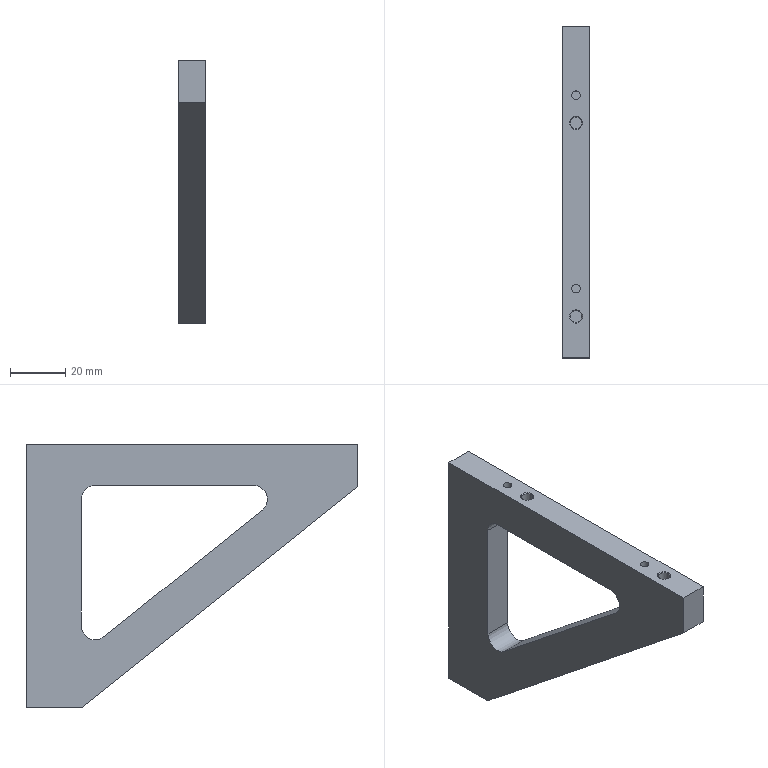Part | STEP file | ROTATION MC_NEW VER-0610_564 | 1 solid | 29 faces | box 10 x 120 x 95.441 mm | volume 51150 mm3 | plane 16 | cylinder 9 | cone 4 | commonest cylinder face diameters 4.2 x4 10 x3 3.03 x2
STEP:
#1=CARTESIAN_POINT('',(-324.569,673.508,-231.532));
#2=VERTEX_POINT('',#1);
#3=CARTESIAN_POINT('',(-322.469,673.508,-231.532));
#4=DIRECTION('',(0.,1.,0.));
#5=DIRECTION('',(-1.,0.,0.));
#6=AXIS2_PLACEMENT_3D('',#3,#4,#5);
#7=CIRCLE('',#6,2.1);
#8=EDGE_CURVE('',#2,#2,#7,.T.);
#9=ORIENTED_EDGE('',*,*,#8,.F.);
#10=CARTESIAN_POINT('',(-324.569,683.208,-231.532));
#11=VERTEX_POINT('',#10);
#12=CARTESIAN_POINT('',(-324.569,688.008,-231.532));
#13=DIRECTION('',(0.,1.,0.));
#14=VECTOR('',#13,2.1);
#15=LINE('',#12,#14);
#16=EDGE_CURVE('',#2,#11,#15,.T.);
#17=ORIENTED_EDGE('',*,*,#16,.T.);
#18=CARTESIAN_POINT('',(-320.369,683.208,-231.532));
#19=VERTEX_POINT('',#18);
#20=CARTESIAN_POINT('',(-322.469,683.208,-231.532));
#21=DIRECTION('',(0.,-1.,0.));
#22=DIRECTION('',(1.,0.,0.));
#23=AXIS2_PLACEMENT_3D('',#20,#21,#22);
#24=CIRCLE('',#23,2.1);
#25=EDGE_CURVE('',#19,#11,#24,.T.);
#26=ORIENTED_EDGE('',*,*,#25,.F.);
#27=CARTESIAN_POINT('',(-322.469,683.208,-231.532));
#28=DIRECTION('',(0.,-1.,0.));
#29=DIRECTION('',(1.,0.,0.));
#30=AXIS2_PLACEMENT_3D('',#27,#28,#29);
#31=CIRCLE('',#30,2.1);
#32=EDGE_CURVE('',#11,#19,#31,.T.);
#33=ORIENTED_EDGE('',*,*,#32,.F.);
#34=ORIENTED_EDGE('',*,*,#16,.F.);
#35=EDGE_LOOP('',(#9,#17,#26,#33,#34));
#36=FACE_OUTER_BOUND('',#35,.T.);
#37=CARTESIAN_POINT('',(-322.469,688.008,-231.532));
#38=DIRECTION('',(0.,1.,0.));
#39=DIRECTION('',(1.,0.,0.));
#40=AXIS2_PLACEMENT_3D('',#37,#38,#39);
#41=CYLINDRICAL_SURFACE('',#40,2.1);
#42=ADVANCED_FACE('',(#36),#41,.F.);
#43=CARTESIAN_POINT('',(-324.569,578.508,-161.091));
#44=VERTEX_POINT('',#43);
#45=CARTESIAN_POINT('',(-320.369,578.508,-161.091));
#46=VERTEX_POINT('',#45);
#47=CARTESIAN_POINT('',(-322.469,578.508,-161.091));
#48=DIRECTION('',(0.,0.,1.));
#49=DIRECTION('',(-1.,0.,0.));
#50=AXIS2_PLACEMENT_3D('',#47,#48,#49);
#51=CIRCLE('',#50,2.1);
#52=EDGE_CURVE('',#44,#46,#51,.T.);
#53=ORIENTED_EDGE('',*,*,#52,.T.);
#54=CARTESIAN_POINT('',(-322.469,578.508,-161.091));
#55=DIRECTION('',(0.,0.,1.));
#56=DIRECTION('',(-1.,0.,0.));
#57=AXIS2_PLACEMENT_3D('',#54,#55,#56);
#58=CIRCLE('',#57,2.1);
#59=EDGE_CURVE('',#46,#44,#58,.T.);
#60=ORIENTED_EDGE('',*,*,#59,.T.);
#61=EDGE_LOOP('',(#53,#60));
#62=FACE_OUTER_BOUND('',#61,.T.);
#63=CARTESIAN_POINT('',(-322.469,623.508,-161.091));
#64=DIRECTION('',(0.,0.,1.));
#65=DIRECTION('',(1.,0.,0.));
#66=AXIS2_PLACEMENT_3D('',#63,#64,#65);
#67=PLANE('',#66);
#68=ADVANCED_FACE('',(#62),#67,.T.);
#69=ORIENTED_EDGE('',*,*,#25,.T.);
#70=ORIENTED_EDGE('',*,*,#32,.T.);
#71=CARTESIAN_POINT('',(-320.069,683.508,-231.532));
#72=VERTEX_POINT('',#71);
#73=CARTESIAN_POINT('',(-321.469,682.108,-231.532));
#74=DIRECTION('',(0.7071,0.7071,0.));
#75=VECTOR('',#74,1.);
#76=LINE('',#73,#75);
#77=EDGE_CURVE('',#19,#72,#76,.T.);
#78=ORIENTED_EDGE('',*,*,#77,.T.);
#79=CARTESIAN_POINT('',(-322.469,683.508,-231.532));
#80=DIRECTION('',(0.,-1.,0.));
#81=DIRECTION('',(-1.,0.,0.));
#82=AXIS2_PLACEMENT_3D('',#79,#80,#81);
#83=CIRCLE('',#82,2.4);
#84=EDGE_CURVE('',#72,#72,#83,.T.);
#85=ORIENTED_EDGE('',*,*,#84,.F.);
#86=ORIENTED_EDGE('',*,*,#77,.F.);
#87=EDGE_LOOP('',(#69,#70,#78,#85,#86));
#88=FACE_OUTER_BOUND('',#87,.T.);
#89=CARTESIAN_POINT('',(-322.469,682.108,-231.532));
#90=DIRECTION('',(0.,1.,0.));
#91=DIRECTION('',(-1.,0.,0.));
#92=AXIS2_PLACEMENT_3D('',#89,#90,#91);
#93=CONICAL_SURFACE('',#92,1.,0.7854);
#94=ADVANCED_FACE('',(#88),#93,.F.);
#95=CARTESIAN_POINT('',(-324.569,578.508,-151.391));
#96=VERTEX_POINT('',#95);
#97=CARTESIAN_POINT('',(-320.369,578.508,-151.391));
#98=VERTEX_POINT('',#97);
#99=CARTESIAN_POINT('',(-322.469,578.508,-151.391));
#100=DIRECTION('',(0.,0.,-1.));
#101=DIRECTION('',(-1.,0.,0.));
#102=AXIS2_PLACEMENT_3D('',#99,#100,#101);
#103=CIRCLE('',#102,2.1);
#104=EDGE_CURVE('',#96,#98,#103,.T.);
#105=ORIENTED_EDGE('',*,*,#104,.F.);
#106=CARTESIAN_POINT('',(-322.469,578.508,-151.391));
#107=DIRECTION('',(0.,0.,-1.));
#108=DIRECTION('',(-1.,0.,0.));
#109=AXIS2_PLACEMENT_3D('',#106,#107,#108);
#110=CIRCLE('',#109,2.1);
#111=EDGE_CURVE('',#98,#96,#110,.T.);
#112=ORIENTED_EDGE('',*,*,#111,.F.);
#113=CARTESIAN_POINT('',(-320.369,578.508,-151.091));
#114=DIRECTION('',(0.,0.,-1.));
#115=VECTOR('',#114,2.1);
#116=LINE('',#113,#115);
#117=EDGE_CURVE('',#98,#46,#116,.T.);
#118=ORIENTED_EDGE('',*,*,#117,.T.);
#119=ORIENTED_EDGE('',*,*,#52,.F.);
#120=ORIENTED_EDGE('',*,*,#59,.F.);
#121=ORIENTED_EDGE('',*,*,#117,.F.);
#122=EDGE_LOOP('',(#105,#112,#118,#119,#120,#121));
#123=FACE_OUTER_BOUND('',#122,.T.);
#124=CARTESIAN_POINT('',(-322.469,578.508,-151.091));
#125=DIRECTION('',(0.,0.,-1.));
#126=DIRECTION('',(-1.,0.,0.));
#127=AXIS2_PLACEMENT_3D('',#124,#125,#126);
#128=CYLINDRICAL_SURFACE('',#127,2.1);
#129=ADVANCED_FACE('',(#123),#128,.F.);
#130=CARTESIAN_POINT('',(-317.469,683.508,-246.532));
#131=VERTEX_POINT('',#130);
#132=CARTESIAN_POINT('',(-327.469,683.508,-246.532));
#133=VERTEX_POINT('',#132);
#134=CARTESIAN_POINT('',(-317.469,683.508,-246.532));
#135=DIRECTION('',(-1.,0.,0.));
#136=VECTOR('',#135,10.);
#137=LINE('',#134,#136);
#138=EDGE_CURVE('',#131,#133,#137,.T.);
#139=ORIENTED_EDGE('',*,*,#138,.T.);
#140=CARTESIAN_POINT('',(-327.469,683.508,-151.091));
#141=VERTEX_POINT('',#140);
#142=CARTESIAN_POINT('',(-327.469,683.508,-151.091));
#143=DIRECTION('',(0.,0.,-1.));
#144=VECTOR('',#143,95.441);
#145=LINE('',#142,#144);
#146=EDGE_CURVE('',#141,#133,#145,.T.);
#147=ORIENTED_EDGE('',*,*,#146,.F.);
#148=CARTESIAN_POINT('',(-317.469,683.508,-151.091));
#149=VERTEX_POINT('',#148);
#150=CARTESIAN_POINT('',(-327.469,683.508,-151.091));
#151=DIRECTION('',(1.,0.,0.));
#152=VECTOR('',#151,10.);
#153=LINE('',#150,#152);
#154=EDGE_CURVE('',#141,#149,#153,.T.);
#155=ORIENTED_EDGE('',*,*,#154,.T.);
#156=CARTESIAN_POINT('',(-317.469,683.508,-151.091));
#157=DIRECTION('',(0.,0.,-1.));
#158=VECTOR('',#157,95.441);
#159=LINE('',#156,#158);
#160=EDGE_CURVE('',#149,#131,#159,.T.);
#161=ORIENTED_EDGE('',*,*,#160,.T.);
#162=EDGE_LOOP('',(#139,#147,#155,#161));
#163=FACE_OUTER_BOUND('',#162,.T.);
#164=CARTESIAN_POINT('',(-320.069,683.508,-163.591));
#165=VERTEX_POINT('',#164);
#166=CARTESIAN_POINT('',(-322.469,683.508,-163.591));
#167=DIRECTION('',(0.,-1.,0.));
#168=DIRECTION('',(1.,0.,0.));
#169=AXIS2_PLACEMENT_3D('',#166,#167,#168);
#170=CIRCLE('',#169,2.4);
#171=EDGE_CURVE('',#165,#165,#170,.T.);
#172=ORIENTED_EDGE('',*,*,#171,.T.);
#173=EDGE_LOOP('',(#172));
#174=FACE_BOUND('',#173,.T.);
#175=ORIENTED_EDGE('',*,*,#84,.T.);
#176=EDGE_LOOP('',(#175));
#177=FACE_BOUND('',#176,.T.);
#178=CARTESIAN_POINT('',(-378.469,683.508,-213.812));
#179=DIRECTION('',(0.,1.,0.));
#180=DIRECTION('',(0.,0.,1.));
#181=AXIS2_PLACEMENT_3D('',#178,#179,#180);
#182=PLANE('',#181);
#183=ADVANCED_FACE('',(#163,#174,#177),#182,.T.);
#184=CARTESIAN_POINT('',(-317.469,663.508,-246.532));
#185=VERTEX_POINT('',#184);
#186=CARTESIAN_POINT('',(-327.469,663.508,-246.532));
#187=VERTEX_POINT('',#186);
#188=CARTESIAN_POINT('',(-317.469,663.508,-246.532));
#189=DIRECTION('',(-1.,0.,0.));
#190=VECTOR('',#189,10.);
#191=LINE('',#188,#190);
#192=EDGE_CURVE('',#185,#187,#191,.T.);
#193=ORIENTED_EDGE('',*,*,#192,.T.);
#194=CARTESIAN_POINT('',(-327.469,683.508,-246.532));
#195=DIRECTION('',(0.,-1.,0.));
#196=VECTOR('',#195,20.);
#197=LINE('',#194,#196);
#198=EDGE_CURVE('',#133,#187,#197,.T.);
#199=ORIENTED_EDGE('',*,*,#198,.F.);
#200=ORIENTED_EDGE('',*,*,#138,.F.);
#201=CARTESIAN_POINT('',(-317.469,683.508,-246.532));
#202=DIRECTION('',(0.,-1.,0.));
#203=VECTOR('',#202,20.);
#204=LINE('',#201,#203);
#205=EDGE_CURVE('',#131,#185,#204,.T.);
#206=ORIENTED_EDGE('',*,*,#205,.T.);
#207=EDGE_LOOP('',(#193,#199,#200,#206));
#208=FACE_OUTER_BOUND('',#207,.T.);
#209=CARTESIAN_POINT('',(-379.469,676.508,-246.532));
#210=DIRECTION('',(0.,0.,-1.));
#211=DIRECTION('',(-1.,0.,0.));
#212=AXIS2_PLACEMENT_3D('',#209,#210,#211);
#213=PLANE('',#212);
#214=ADVANCED_FACE('',(#208),#213,.T.);
#215=CARTESIAN_POINT('',(-327.469,563.508,-166.532));
#216=VERTEX_POINT('',#215);
#217=CARTESIAN_POINT('',(-327.469,663.508,-246.532));
#218=DIRECTION('',(0.,-0.7809,0.6247));
#219=VECTOR('',#218,128.062);
#220=LINE('',#217,#219);
#221=EDGE_CURVE('',#187,#216,#220,.T.);
#222=ORIENTED_EDGE('',*,*,#221,.F.);
#223=ORIENTED_EDGE('',*,*,#192,.F.);
#224=CARTESIAN_POINT('',(-317.469,563.508,-166.532));
#225=VERTEX_POINT('',#224);
#226=CARTESIAN_POINT('',(-317.469,563.508,-166.532));
#227=DIRECTION('',(0.,0.7809,-0.6247));
#228=VECTOR('',#227,128.062);
#229=LINE('',#226,#228);
#230=EDGE_CURVE('',#225,#185,#229,.T.);
#231=ORIENTED_EDGE('',*,*,#230,.F.);
#232=CARTESIAN_POINT('',(-327.469,563.508,-166.532));
#233=DIRECTION('',(1.,0.,0.));
#234=VECTOR('',#233,10.);
#235=LINE('',#232,#234);
#236=EDGE_CURVE('',#216,#225,#235,.T.);
#237=ORIENTED_EDGE('',*,*,#236,.F.);
#238=EDGE_LOOP('',(#222,#223,#231,#237));
#239=FACE_OUTER_BOUND('',#238,.T.);
#240=CARTESIAN_POINT('',(-378.969,613.508,-206.532));
#241=DIRECTION('',(0.,-0.6247,-0.7809));
#242=DIRECTION('',(-1.,0.,0.));
#243=AXIS2_PLACEMENT_3D('',#240,#241,#242);
#244=PLANE('',#243);
#245=ADVANCED_FACE('',(#239),#244,.T.);
#246=ORIENTED_EDGE('',*,*,#221,.T.);
#247=CARTESIAN_POINT('',(-327.469,563.508,-151.091));
#248=VERTEX_POINT('',#247);
#249=CARTESIAN_POINT('',(-327.469,563.508,-151.091));
#250=DIRECTION('',(0.,0.,-1.));
#251=VECTOR('',#250,15.441);
#252=LINE('',#249,#251);
#253=EDGE_CURVE('',#248,#216,#252,.T.);
#254=ORIENTED_EDGE('',*,*,#253,.F.);
#255=CARTESIAN_POINT('',(-327.469,563.508,-151.091));
#256=DIRECTION('',(0.,1.,0.));
#257=VECTOR('',#256,120.);
#258=LINE('',#255,#257);
#259=EDGE_CURVE('',#248,#141,#258,.T.);
#260=ORIENTED_EDGE('',*,*,#259,.T.);
#261=ORIENTED_EDGE('',*,*,#146,.T.);
#262=ORIENTED_EDGE('',*,*,#198,.T.);
#263=EDGE_LOOP('',(#246,#254,#260,#261,#262));
#264=FACE_OUTER_BOUND('',#263,.T.);
#265=CARTESIAN_POINT('',(-327.469,601.223,-166.091));
#266=VERTEX_POINT('',#265);
#267=CARTESIAN_POINT('',(-327.469,598.099,-174.996));
#268=VERTEX_POINT('',#267);
#269=CARTESIAN_POINT('',(-327.469,601.223,-171.091));
#270=DIRECTION('',(1.,0.,0.));
#271=DIRECTION('',(0.,-0.9436,0.331));
#272=AXIS2_PLACEMENT_3D('',#269,#270,#271);
#273=CIRCLE('',#272,5.);
#274=EDGE_CURVE('',#266,#268,#273,.T.);
#275=ORIENTED_EDGE('',*,*,#274,.T.);
#276=CARTESIAN_POINT('',(-327.469,655.385,-220.824));
#277=VERTEX_POINT('',#276);
#278=CARTESIAN_POINT('',(-327.469,598.099,-174.996));
#279=DIRECTION('',(0.,0.7809,-0.6247));
#280=VECTOR('',#279,73.361);
#281=LINE('',#278,#280);
#282=EDGE_CURVE('',#268,#277,#281,.T.);
#283=ORIENTED_EDGE('',*,*,#282,.T.);
#284=CARTESIAN_POINT('',(-327.469,663.508,-216.92));
#285=VERTEX_POINT('',#284);
#286=CARTESIAN_POINT('',(-327.469,658.508,-216.92));
#287=DIRECTION('',(1.,0.,0.));
#288=DIRECTION('',(0.,-0.6247,-0.7809));
#289=AXIS2_PLACEMENT_3D('',#286,#287,#288);
#290=CIRCLE('',#289,5.);
#291=EDGE_CURVE('',#277,#285,#290,.T.);
#292=ORIENTED_EDGE('',*,*,#291,.T.);
#293=CARTESIAN_POINT('',(-327.469,663.508,-171.091));
#294=VERTEX_POINT('',#293);
#295=CARTESIAN_POINT('',(-327.469,663.508,-171.091));
#296=DIRECTION('',(0.,0.,-1.));
#297=VECTOR('',#296,45.829);
#298=LINE('',#295,#297);
#299=EDGE_CURVE('',#294,#285,#298,.T.);
#300=ORIENTED_EDGE('',*,*,#299,.F.);
#301=CARTESIAN_POINT('',(-327.469,658.508,-166.091));
#302=VERTEX_POINT('',#301);
#303=CARTESIAN_POINT('',(-327.469,658.508,-171.091));
#304=DIRECTION('',(1.,0.,0.));
#305=DIRECTION('',(0.,1.,0.));
#306=AXIS2_PLACEMENT_3D('',#303,#304,#305);
#307=CIRCLE('',#306,5.);
#308=EDGE_CURVE('',#294,#302,#307,.T.);
#309=ORIENTED_EDGE('',*,*,#308,.T.);
#310=CARTESIAN_POINT('',(-327.469,601.223,-166.091));
#311=DIRECTION('',(0.,1.,0.));
#312=VECTOR('',#311,57.286);
#313=LINE('',#310,#312);
#314=EDGE_CURVE('',#266,#302,#313,.T.);
#315=ORIENTED_EDGE('',*,*,#314,.F.);
#316=EDGE_LOOP('',(#275,#283,#292,#300,#309,#315));
#317=FACE_BOUND('',#316,.T.);
#318=CARTESIAN_POINT('',(-327.469,683.508,-213.812));
#319=DIRECTION('',(-1.,0.,0.));
#320=DIRECTION('',(0.,0.,1.));
#321=AXIS2_PLACEMENT_3D('',#318,#319,#320);
#322=PLANE('',#321);
#323=ADVANCED_FACE('',(#264,#317),#322,.T.);
#324=ORIENTED_EDGE('',*,*,#154,.F.);
#325=ORIENTED_EDGE('',*,*,#259,.F.);
#326=CARTESIAN_POINT('',(-317.469,563.508,-151.091));
#327=VERTEX_POINT('',#326);
#328=CARTESIAN_POINT('',(-327.469,563.508,-151.091));
#329=DIRECTION('',(1.,0.,0.));
#330=VECTOR('',#329,10.);
#331=LINE('',#328,#330);
#332=EDGE_CURVE('',#248,#327,#331,.T.);
#333=ORIENTED_EDGE('',*,*,#332,.T.);
#334=CARTESIAN_POINT('',(-317.469,683.508,-151.091));
#335=DIRECTION('',(0.,-1.,0.));
#336=VECTOR('',#335,120.);
#337=LINE('',#334,#336);
#338=EDGE_CURVE('',#149,#327,#337,.T.);
#339=ORIENTED_EDGE('',*,*,#338,.F.);
#340=EDGE_LOOP('',(#324,#325,#333,#339));
#341=FACE_OUTER_BOUND('',#340,.T.);
#342=CARTESIAN_POINT('',(-320.069,648.508,-151.091));
#343=VERTEX_POINT('',#342);
#344=CARTESIAN_POINT('',(-324.869,648.508,-151.091));
#345=VERTEX_POINT('',#344);
#346=CARTESIAN_POINT('',(-322.469,648.508,-151.091));
#347=DIRECTION('',(0.,0.,-1.));
#348=DIRECTION('',(-1.,0.,0.));
#349=AXIS2_PLACEMENT_3D('',#346,#347,#348);
#350=CIRCLE('',#349,2.4);
#351=EDGE_CURVE('',#343,#345,#350,.T.);
#352=ORIENTED_EDGE('',*,*,#351,.T.);
#353=CARTESIAN_POINT('',(-322.469,648.508,-151.091));
#354=DIRECTION('',(0.,0.,-1.));
#355=DIRECTION('',(-1.,0.,0.));
#356=AXIS2_PLACEMENT_3D('',#353,#354,#355);
#357=CIRCLE('',#356,2.4);
#358=EDGE_CURVE('',#345,#343,#357,.T.);
#359=ORIENTED_EDGE('',*,*,#358,.T.);
#360=EDGE_LOOP('',(#352,#359));
#361=FACE_BOUND('',#360,.T.);
#362=CARTESIAN_POINT('',(-320.069,578.508,-151.091));
#363=VERTEX_POINT('',#362);
#364=CARTESIAN_POINT('',(-324.869,578.508,-151.091));
#365=VERTEX_POINT('',#364);
#366=CARTESIAN_POINT('',(-322.469,578.508,-151.091));
#367=DIRECTION('',(0.,0.,-1.));
#368=DIRECTION('',(-1.,0.,0.));
#369=AXIS2_PLACEMENT_3D('',#366,#367,#368);
#370=CIRCLE('',#369,2.4);
#371=EDGE_CURVE('',#363,#365,#370,.T.);
#372=ORIENTED_EDGE('',*,*,#371,.T.);
#373=CARTESIAN_POINT('',(-322.469,578.508,-151.091));
#374=DIRECTION('',(0.,0.,-1.));
#375=DIRECTION('',(-1.,0.,0.));
#376=AXIS2_PLACEMENT_3D('',#373,#374,#375);
#377=CIRCLE('',#376,2.4);
#378=EDGE_CURVE('',#365,#363,#377,.T.);
#379=ORIENTED_EDGE('',*,*,#378,.T.);
#380=EDGE_LOOP('',(#372,#379));
#381=FACE_BOUND('',#380,.T.);
#382=CARTESIAN_POINT('',(-320.954,588.508,-151.091));
#383=VERTEX_POINT('',#382);
#384=CARTESIAN_POINT('',(-323.984,588.508,-151.091));
#385=VERTEX_POINT('',#384);
#386=CARTESIAN_POINT('',(-322.469,588.508,-151.091));
#387=DIRECTION('',(0.,0.,1.));
#388=DIRECTION('',(1.,0.,0.));
#389=AXIS2_PLACEMENT_3D('',#386,#387,#388);
#390=CIRCLE('',#389,1.515);
#391=EDGE_CURVE('',#383,#385,#390,.T.);
#392=ORIENTED_EDGE('',*,*,#391,.F.);
#393=CARTESIAN_POINT('',(-322.469,588.508,-151.091));
#394=DIRECTION('',(0.,0.,1.));
#395=DIRECTION('',(1.,0.,0.));
#396=AXIS2_PLACEMENT_3D('',#393,#394,#395);
#397=CIRCLE('',#396,1.515);
#398=EDGE_CURVE('',#385,#383,#397,.T.);
#399=ORIENTED_EDGE('',*,*,#398,.F.);
#400=EDGE_LOOP('',(#392,#399));
#401=FACE_BOUND('',#400,.T.);
#402=CARTESIAN_POINT('',(-320.954,658.508,-151.091));
#403=VERTEX_POINT('',#402);
#404=CARTESIAN_POINT('',(-323.984,658.508,-151.091));
#405=VERTEX_POINT('',#404);
#406=CARTESIAN_POINT('',(-322.469,658.508,-151.091));
#407=DIRECTION('',(0.,0.,1.));
#408=DIRECTION('',(1.,0.,0.));
#409=AXIS2_PLACEMENT_3D('',#406,#407,#408);
#410=CIRCLE('',#409,1.515);
#411=EDGE_CURVE('',#403,#405,#410,.T.);
#412=ORIENTED_EDGE('',*,*,#411,.F.);
#413=CARTESIAN_POINT('',(-322.469,658.508,-151.091));
#414=DIRECTION('',(0.,0.,1.));
#415=DIRECTION('',(1.,0.,0.));
#416=AXIS2_PLACEMENT_3D('',#413,#414,#415);
#417=CIRCLE('',#416,1.515);
#418=EDGE_CURVE('',#405,#403,#417,.T.);
#419=ORIENTED_EDGE('',*,*,#418,.F.);
#420=EDGE_LOOP('',(#412,#419));
#421=FACE_BOUND('',#420,.T.);
#422=CARTESIAN_POINT('',(-379.469,676.508,-151.091));
#423=DIRECTION('',(0.,0.,1.));
#424=DIRECTION('',(1.,0.,0.));
#425=AXIS2_PLACEMENT_3D('',#422,#423,#424);
#426=PLANE('',#425);
#427=ADVANCED_FACE('',(#341,#361,#381,#401,#421),#426,.T.);
#428=ORIENTED_EDGE('',*,*,#230,.T.);
#429=ORIENTED_EDGE('',*,*,#205,.F.);
#430=ORIENTED_EDGE('',*,*,#160,.F.);
#431=ORIENTED_EDGE('',*,*,#338,.T.);
#432=CARTESIAN_POINT('',(-317.469,563.508,-151.091));
#433=DIRECTION('',(0.,0.,-1.));
#434=VECTOR('',#433,15.441);
#435=LINE('',#432,#434);
#436=EDGE_CURVE('',#327,#225,#435,.T.);
#437=ORIENTED_EDGE('',*,*,#436,.T.);
#438=EDGE_LOOP('',(#428,#429,#430,#431,#437));
#439=FACE_OUTER_BOUND('',#438,.T.);
#440=CARTESIAN_POINT('',(-317.469,663.508,-216.92));
#441=VERTEX_POINT('',#440);
#442=CARTESIAN_POINT('',(-317.469,663.508,-171.091));
#443=VERTEX_POINT('',#442);
#444=CARTESIAN_POINT('',(-317.469,663.508,-216.92));
#445=DIRECTION('',(0.,0.,1.));
#446=VECTOR('',#445,45.829);
#447=LINE('',#444,#446);
#448=EDGE_CURVE('',#441,#443,#447,.T.);
#449=ORIENTED_EDGE('',*,*,#448,.F.);
#450=CARTESIAN_POINT('',(-317.469,655.385,-220.824));
#451=VERTEX_POINT('',#450);
#452=CARTESIAN_POINT('',(-317.469,658.508,-216.92));
#453=DIRECTION('',(-1.,0.,0.));
#454=DIRECTION('',(0.,1.,0.));
#455=AXIS2_PLACEMENT_3D('',#452,#453,#454);
#456=CIRCLE('',#455,5.);
#457=EDGE_CURVE('',#441,#451,#456,.T.);
#458=ORIENTED_EDGE('',*,*,#457,.T.);
#459=CARTESIAN_POINT('',(-317.469,598.099,-174.996));
#460=VERTEX_POINT('',#459);
#461=CARTESIAN_POINT('',(-317.469,655.385,-220.824));
#462=DIRECTION('',(0.,-0.7809,0.6247));
#463=VECTOR('',#462,73.361);
#464=LINE('',#461,#463);
#465=EDGE_CURVE('',#451,#460,#464,.T.);
#466=ORIENTED_EDGE('',*,*,#465,.T.);
#467=CARTESIAN_POINT('',(-317.469,601.223,-166.091));
#468=VERTEX_POINT('',#467);
#469=CARTESIAN_POINT('',(-317.469,601.223,-171.091));
#470=DIRECTION('',(-1.,0.,0.));
#471=DIRECTION('',(0.,-0.6247,-0.7809));
#472=AXIS2_PLACEMENT_3D('',#469,#470,#471);
#473=CIRCLE('',#472,5.);
#474=EDGE_CURVE('',#460,#468,#473,.T.);
#475=ORIENTED_EDGE('',*,*,#474,.T.);
#476=CARTESIAN_POINT('',(-317.469,658.508,-166.091));
#477=VERTEX_POINT('',#476);
#478=CARTESIAN_POINT('',(-317.469,658.508,-166.091));
#479=DIRECTION('',(0.,-1.,0.));
#480=VECTOR('',#479,57.286);
#481=LINE('',#478,#480);
#482=EDGE_CURVE('',#477,#468,#481,.T.);
#483=ORIENTED_EDGE('',*,*,#482,.F.);
#484=CARTESIAN_POINT('',(-317.469,658.508,-171.091));
#485=DIRECTION('',(-1.,0.,0.));
#486=DIRECTION('',(0.,0.,1.));
#487=AXIS2_PLACEMENT_3D('',#484,#485,#486);
#488=CIRCLE('',#487,5.);
#489=EDGE_CURVE('',#477,#443,#488,.T.);
#490=ORIENTED_EDGE('',*,*,#489,.T.);
#491=EDGE_LOOP('',(#449,#458,#466,#475,#483,#490));
#492=FACE_BOUND('',#491,.T.);
#493=CARTESIAN_POINT('',(-317.469,676.508,-213.812));
#494=DIRECTION('',(1.,0.,0.));
#495=DIRECTION('',(0.,0.,-1.));
#496=AXIS2_PLACEMENT_3D('',#493,#494,#495);
#497=PLANE('',#496);
#498=ADVANCED_FACE('',(#439,#492),#497,.T.);
#499=ORIENTED_EDGE('',*,*,#236,.T.);
#500=ORIENTED_EDGE('',*,*,#436,.F.);
#501=ORIENTED_EDGE('',*,*,#332,.F.);
#502=ORIENTED_EDGE('',*,*,#253,.T.);
#503=EDGE_LOOP('',(#499,#500,#501,#502));
#504=FACE_OUTER_BOUND('',#503,.T.);
#505=CARTESIAN_POINT('',(-378.469,563.508,-213.812));
#506=DIRECTION('',(0.,1.,0.));
#507=DIRECTION('',(0.,0.,1.));
#508=AXIS2_PLACEMENT_3D('',#505,#506,#507);
#509=PLANE('',#508);
#510=ADVANCED_FACE('',(#504),#509,.F.);
#511=CARTESIAN_POINT('',(-317.469,663.508,-216.92));
#512=DIRECTION('',(-1.,0.,0.));
#513=VECTOR('',#512,10.);
#514=LINE('',#511,#513);
#515=EDGE_CURVE('',#441,#285,#514,.T.);
#516=ORIENTED_EDGE('',*,*,#515,.F.);
#517=ORIENTED_EDGE('',*,*,#448,.T.);
#518=CARTESIAN_POINT('',(-327.469,663.508,-171.091));
#519=DIRECTION('',(1.,0.,0.));
#520=VECTOR('',#519,10.);
#521=LINE('',#518,#520);
#522=EDGE_CURVE('',#294,#443,#521,.T.);
#523=ORIENTED_EDGE('',*,*,#522,.F.);
#524=ORIENTED_EDGE('',*,*,#299,.T.);
#525=EDGE_LOOP('',(#516,#517,#523,#524));
#526=FACE_OUTER_BOUND('',#525,.T.);
#527=CARTESIAN_POINT('',(-317.469,663.508,-198.707));
#528=DIRECTION('',(0.,1.,0.));
#529=DIRECTION('',(0.,0.,1.));
#530=AXIS2_PLACEMENT_3D('',#527,#528,#529);
#531=PLANE('',#530);
#532=ADVANCED_FACE('',(#526),#531,.F.);
#533=ORIENTED_EDGE('',*,*,#457,.F.);
#534=ORIENTED_EDGE('',*,*,#515,.T.);
#535=ORIENTED_EDGE('',*,*,#291,.F.);
#536=CARTESIAN_POINT('',(-327.469,655.385,-220.824));
#537=DIRECTION('',(1.,0.,0.));
#538=VECTOR('',#537,10.);
#539=LINE('',#536,#538);
#540=EDGE_CURVE('',#277,#451,#539,.T.);
#541=ORIENTED_EDGE('',*,*,#540,.T.);
#542=EDGE_LOOP('',(#533,#534,#535,#541));
#543=FACE_OUTER_BOUND('',#542,.T.);
#544=CARTESIAN_POINT('',(-317.469,658.508,-216.92));
#545=DIRECTION('',(-1.,0.,0.));
#546=DIRECTION('',(0.,0.4332,-0.9013));
#547=AXIS2_PLACEMENT_3D('',#544,#545,#546);
#548=CYLINDRICAL_SURFACE('',#547,5.);
#549=ADVANCED_FACE('',(#543),#548,.F.);
#550=CARTESIAN_POINT('',(-324.569,673.508,-163.591));
#551=VERTEX_POINT('',#550);
#552=CARTESIAN_POINT('',(-322.469,673.508,-163.591));
#553=DIRECTION('',(0.,1.,0.));
#554=DIRECTION('',(1.,0.,0.));
#555=AXIS2_PLACEMENT_3D('',#552,#553,#554);
#556=CIRCLE('',#555,2.1);
#557=EDGE_CURVE('',#551,#551,#556,.T.);
#558=ORIENTED_EDGE('',*,*,#557,.T.);
#559=EDGE_LOOP('',(#558));
#560=FACE_OUTER_BOUND('',#559,.T.);
#561=CARTESIAN_POINT('',(-378.469,673.508,-213.812));
#562=DIRECTION('',(0.,1.,0.));
#563=DIRECTION('',(0.,0.,1.));
#564=AXIS2_PLACEMENT_3D('',#561,#562,#563);
#565=PLANE('',#564);
#566=ADVANCED_FACE('',(#560),#565,.T.);
#567=ORIENTED_EDGE('',*,*,#540,.F.);
#568=ORIENTED_EDGE('',*,*,#282,.F.);
#569=CARTESIAN_POINT('',(-317.469,598.099,-174.996));
#570=DIRECTION('',(-1.,0.,0.));
#571=VECTOR('',#570,10.);
#572=LINE('',#569,#571);
#573=EDGE_CURVE('',#460,#268,#572,.T.);
#574=ORIENTED_EDGE('',*,*,#573,.F.);
#575=ORIENTED_EDGE('',*,*,#465,.F.);
#576=EDGE_LOOP('',(#567,#568,#574,#575));
#577=FACE_OUTER_BOUND('',#576,.T.);
#578=CARTESIAN_POINT('',(-317.469,627.739,-198.707));
#579=DIRECTION('',(0.,-0.6247,-0.7809));
#580=DIRECTION('',(-1.,0.,0.));
#581=AXIS2_PLACEMENT_3D('',#578,#579,#580);
#582=PLANE('',#581);
#583=ADVANCED_FACE('',(#577),#582,.F.);
#584=ORIENTED_EDGE('',*,*,#274,.F.);
#585=CARTESIAN_POINT('',(-327.469,601.223,-166.091));
#586=DIRECTION('',(1.,0.,0.));
#587=VECTOR('',#586,10.);
#588=LINE('',#585,#587);
#589=EDGE_CURVE('',#266,#468,#588,.T.);
#590=ORIENTED_EDGE('',*,*,#589,.T.);
#591=ORIENTED_EDGE('',*,*,#474,.F.);
#592=ORIENTED_EDGE('',*,*,#573,.T.);
#593=EDGE_LOOP('',(#584,#590,#591,#592));
#594=FACE_OUTER_BOUND('',#593,.T.);
#595=CARTESIAN_POINT('',(-317.469,601.223,-171.091));
#596=DIRECTION('',(1.,0.,0.));
#597=DIRECTION('',(0.,-0.9436,0.331));
#598=AXIS2_PLACEMENT_3D('',#595,#596,#597);
#599=CYLINDRICAL_SURFACE('',#598,5.);
#600=ADVANCED_FACE('',(#594),#599,.F.);
#601=ORIENTED_EDGE('',*,*,#8,.T.);
#602=EDGE_LOOP('',(#601));
#603=FACE_OUTER_BOUND('',#602,.T.);
#604=CARTESIAN_POINT('',(-378.469,673.508,-243.802));
#605=DIRECTION('',(0.,1.,0.));
#606=DIRECTION('',(0.,0.,1.));
#607=AXIS2_PLACEMENT_3D('',#604,#605,#606);
#608=PLANE('',#607);
#609=ADVANCED_FACE('',(#603),#608,.T.);
#610=CARTESIAN_POINT('',(-317.469,658.508,-166.091));
#611=DIRECTION('',(-1.,0.,0.));
#612=VECTOR('',#611,10.);
#613=LINE('',#610,#612);
#614=EDGE_CURVE('',#477,#302,#613,.T.);
#615=ORIENTED_EDGE('',*,*,#614,.F.);
#616=ORIENTED_EDGE('',*,*,#482,.T.);
#617=ORIENTED_EDGE('',*,*,#589,.F.);
#618=ORIENTED_EDGE('',*,*,#314,.T.);
#619=EDGE_LOOP('',(#615,#616,#617,#618));
#620=FACE_OUTER_BOUND('',#619,.T.);
#621=CARTESIAN_POINT('',(-317.469,627.739,-166.091));
#622=DIRECTION('',(0.,0.,1.));
#623=DIRECTION('',(1.,0.,0.));
#624=AXIS2_PLACEMENT_3D('',#621,#622,#623);
#625=PLANE('',#624);
#626=ADVANCED_FACE('',(#620),#625,.F.);
#627=ORIENTED_EDGE('',*,*,#489,.F.);
#628=ORIENTED_EDGE('',*,*,#614,.T.);
#629=ORIENTED_EDGE('',*,*,#308,.F.);
#630=ORIENTED_EDGE('',*,*,#522,.T.);
#631=EDGE_LOOP('',(#627,#628,#629,#630));
#632=FACE_OUTER_BOUND('',#631,.T.);
#633=CARTESIAN_POINT('',(-317.469,658.508,-171.091));
#634=DIRECTION('',(-1.,0.,0.));
#635=DIRECTION('',(0.,0.7071,0.7071));
#636=AXIS2_PLACEMENT_3D('',#633,#634,#635);
#637=CYLINDRICAL_SURFACE('',#636,5.);
#638=ADVANCED_FACE('',(#632),#637,.F.);
#639=ORIENTED_EDGE('',*,*,#104,.T.);
#640=ORIENTED_EDGE('',*,*,#111,.T.);
#641=CARTESIAN_POINT('',(-323.469,578.508,-152.491));
#642=DIRECTION('',(-0.7071,0.,0.7071));
#643=VECTOR('',#642,1.);
#644=LINE('',#641,#643);
#645=EDGE_CURVE('',#96,#365,#644,.T.);
#646=ORIENTED_EDGE('',*,*,#645,.T.);
#647=ORIENTED_EDGE('',*,*,#371,.F.);
#648=ORIENTED_EDGE('',*,*,#378,.F.);
#649=ORIENTED_EDGE('',*,*,#645,.F.);
#650=EDGE_LOOP('',(#639,#640,#646,#647,#648,#649));
#651=FACE_OUTER_BOUND('',#650,.T.);
#652=CARTESIAN_POINT('',(-322.469,578.508,-152.491));
#653=DIRECTION('',(0.,0.,1.));
#654=DIRECTION('',(1.,0.,0.));
#655=AXIS2_PLACEMENT_3D('',#652,#653,#654);
#656=CONICAL_SURFACE('',#655,1.,0.7854);
#657=ADVANCED_FACE('',(#651),#656,.F.);
#658=CARTESIAN_POINT('',(-320.369,648.508,-151.391));
#659=VERTEX_POINT('',#658);
#660=CARTESIAN_POINT('',(-324.569,648.508,-151.391));
#661=VERTEX_POINT('',#660);
#662=CARTESIAN_POINT('',(-322.469,648.508,-151.391));
#663=DIRECTION('',(0.,0.,-1.));
#664=DIRECTION('',(-1.,0.,0.));
#665=AXIS2_PLACEMENT_3D('',#662,#663,#664);
#666=CIRCLE('',#665,2.1);
#667=EDGE_CURVE('',#659,#661,#666,.T.);
#668=ORIENTED_EDGE('',*,*,#667,.T.);
#669=CARTESIAN_POINT('',(-323.469,648.508,-152.491));
#670=DIRECTION('',(-0.7071,0.,0.7071));
#671=VECTOR('',#670,1.);
#672=LINE('',#669,#671);
#673=EDGE_CURVE('',#661,#345,#672,.T.);
#674=ORIENTED_EDGE('',*,*,#673,.T.);
#675=ORIENTED_EDGE('',*,*,#351,.F.);
#676=ORIENTED_EDGE('',*,*,#358,.F.);
#677=ORIENTED_EDGE('',*,*,#673,.F.);
#678=CARTESIAN_POINT('',(-322.469,648.508,-151.391));
#679=DIRECTION('',(0.,0.,-1.));
#680=DIRECTION('',(-1.,0.,0.));
#681=AXIS2_PLACEMENT_3D('',#678,#679,#680);
#682=CIRCLE('',#681,2.1);
#683=EDGE_CURVE('',#661,#659,#682,.T.);
#684=ORIENTED_EDGE('',*,*,#683,.T.);
#685=EDGE_LOOP('',(#668,#674,#675,#676,#677,#684));
#686=FACE_OUTER_BOUND('',#685,.T.);
#687=CARTESIAN_POINT('',(-322.469,648.508,-152.491));
#688=DIRECTION('',(0.,0.,1.));
#689=DIRECTION('',(1.,0.,0.));
#690=AXIS2_PLACEMENT_3D('',#687,#688,#689);
#691=CONICAL_SURFACE('',#690,1.,0.7854);
#692=ADVANCED_FACE('',(#686),#691,.F.);
#693=ORIENTED_EDGE('',*,*,#557,.F.);
#694=CARTESIAN_POINT('',(-324.569,683.208,-163.591));
#695=VERTEX_POINT('',#694);
#696=CARTESIAN_POINT('',(-324.569,688.008,-163.591));
#697=DIRECTION('',(0.,1.,0.));
#698=VECTOR('',#697,2.1);
#699=LINE('',#696,#698);
#700=EDGE_CURVE('',#551,#695,#699,.T.);
#701=ORIENTED_EDGE('',*,*,#700,.T.);
#702=CARTESIAN_POINT('',(-320.369,683.208,-163.591));
#703=VERTEX_POINT('',#702);
#704=CARTESIAN_POINT('',(-322.469,683.208,-163.591));
#705=DIRECTION('',(0.,-1.,0.));
#706=DIRECTION('',(1.,0.,0.));
#707=AXIS2_PLACEMENT_3D('',#704,#705,#706);
#708=CIRCLE('',#707,2.1);
#709=EDGE_CURVE('',#703,#695,#708,.T.);
#710=ORIENTED_EDGE('',*,*,#709,.F.);
#711=CARTESIAN_POINT('',(-322.469,683.208,-163.591));
#712=DIRECTION('',(0.,-1.,0.));
#713=DIRECTION('',(1.,0.,0.));
#714=AXIS2_PLACEMENT_3D('',#711,#712,#713);
#715=CIRCLE('',#714,2.1);
#716=EDGE_CURVE('',#695,#703,#715,.T.);
#717=ORIENTED_EDGE('',*,*,#716,.F.);
#718=ORIENTED_EDGE('',*,*,#700,.F.);
#719=EDGE_LOOP('',(#693,#701,#710,#717,#718));
#720=FACE_OUTER_BOUND('',#719,.T.);
#721=CARTESIAN_POINT('',(-322.469,688.008,-163.591));
#722=DIRECTION('',(0.,1.,0.));
#723=DIRECTION('',(1.,0.,0.));
#724=AXIS2_PLACEMENT_3D('',#721,#722,#723);
#725=CYLINDRICAL_SURFACE('',#724,2.1);
#726=ADVANCED_FACE('',(#720),#725,.F.);
#727=ORIENTED_EDGE('',*,*,#667,.F.);
#728=CARTESIAN_POINT('',(-320.369,648.508,-161.091));
#729=VERTEX_POINT('',#728);
#730=CARTESIAN_POINT('',(-320.369,648.508,-151.091));
#731=DIRECTION('',(0.,0.,-1.));
#732=VECTOR('',#731,2.1);
#733=LINE('',#730,#732);
#734=EDGE_CURVE('',#659,#729,#733,.T.);
#735=ORIENTED_EDGE('',*,*,#734,.T.);
#736=CARTESIAN_POINT('',(-324.569,648.508,-161.091));
#737=VERTEX_POINT('',#736);
#738=CARTESIAN_POINT('',(-322.469,648.508,-161.091));
#739=DIRECTION('',(0.,0.,1.));
#740=DIRECTION('',(-1.,0.,0.));
#741=AXIS2_PLACEMENT_3D('',#738,#739,#740);
#742=CIRCLE('',#741,2.1);
#743=EDGE_CURVE('',#737,#729,#742,.T.);
#744=ORIENTED_EDGE('',*,*,#743,.F.);
#745=CARTESIAN_POINT('',(-322.469,648.508,-161.091));
#746=DIRECTION('',(0.,0.,1.));
#747=DIRECTION('',(-1.,0.,0.));
#748=AXIS2_PLACEMENT_3D('',#745,#746,#747);
#749=CIRCLE('',#748,2.1);
#750=EDGE_CURVE('',#729,#737,#749,.T.);
#751=ORIENTED_EDGE('',*,*,#750,.F.);
#752=ORIENTED_EDGE('',*,*,#734,.F.);
#753=ORIENTED_EDGE('',*,*,#683,.F.);
#754=EDGE_LOOP('',(#727,#735,#744,#751,#752,#753));
#755=FACE_OUTER_BOUND('',#754,.T.);
#756=CARTESIAN_POINT('',(-322.469,648.508,-151.091));
#757=DIRECTION('',(0.,0.,-1.));
#758=DIRECTION('',(-1.,0.,0.));
#759=AXIS2_PLACEMENT_3D('',#756,#757,#758);
#760=CYLINDRICAL_SURFACE('',#759,2.1);
#761=ADVANCED_FACE('',(#755),#760,.F.);
#762=ORIENTED_EDGE('',*,*,#709,.T.);
#763=ORIENTED_EDGE('',*,*,#716,.T.);
#764=CARTESIAN_POINT('',(-321.469,682.108,-163.591));
#765=DIRECTION('',(0.7071,0.7071,0.));
#766=VECTOR('',#765,1.);
#767=LINE('',#764,#766);
#768=EDGE_CURVE('',#703,#165,#767,.T.);
#769=ORIENTED_EDGE('',*,*,#768,.T.);
#770=ORIENTED_EDGE('',*,*,#171,.F.);
#771=ORIENTED_EDGE('',*,*,#768,.F.);
#772=EDGE_LOOP('',(#762,#763,#769,#770,#771));
#773=FACE_OUTER_BOUND('',#772,.T.);
#774=CARTESIAN_POINT('',(-322.469,682.108,-163.591));
#775=DIRECTION('',(0.,1.,0.));
#776=DIRECTION('',(-1.,0.,0.));
#777=AXIS2_PLACEMENT_3D('',#774,#775,#776);
#778=CONICAL_SURFACE('',#777,1.,0.7854);
#779=ADVANCED_FACE('',(#773),#778,.F.);
#780=ORIENTED_EDGE('',*,*,#743,.T.);
#781=ORIENTED_EDGE('',*,*,#750,.T.);
#782=EDGE_LOOP('',(#780,#781));
#783=FACE_OUTER_BOUND('',#782,.T.);
#784=CARTESIAN_POINT('',(-322.469,623.508,-161.091));
#785=DIRECTION('',(0.,0.,1.));
#786=DIRECTION('',(1.,0.,0.));
#787=AXIS2_PLACEMENT_3D('',#784,#785,#786);
#788=PLANE('',#787);
#789=ADVANCED_FACE('',(#783),#788,.T.);
#790=CARTESIAN_POINT('',(-323.984,658.508,-157.091));
#791=VERTEX_POINT('',#790);
#792=CARTESIAN_POINT('',(-322.469,658.508,-157.091));
#793=DIRECTION('',(0.,0.,1.));
#794=DIRECTION('',(-1.,0.,0.));
#795=AXIS2_PLACEMENT_3D('',#792,#793,#794);
#796=CIRCLE('',#795,1.515);
#797=EDGE_CURVE('',#791,#791,#796,.F.);
#798=ORIENTED_EDGE('',*,*,#797,.F.);
#799=EDGE_LOOP('',(#798));
#800=FACE_OUTER_BOUND('',#799,.T.);
#801=CARTESIAN_POINT('',(-322.469,658.508,-157.091));
#802=DIRECTION('',(0.,0.,-1.));
#803=DIRECTION('',(-1.,0.,0.));
#804=AXIS2_PLACEMENT_3D('',#801,#802,#803);
#805=PLANE('',#804);
#806=ADVANCED_FACE('',(#800),#805,.F.);
#807=ORIENTED_EDGE('',*,*,#797,.T.);
#808=CARTESIAN_POINT('',(-323.984,658.508,-151.091));
#809=DIRECTION('',(0.,0.,1.));
#810=VECTOR('',#809,1.515);
#811=LINE('',#808,#810);
#812=EDGE_CURVE('',#791,#405,#811,.T.);
#813=ORIENTED_EDGE('',*,*,#812,.T.);
#814=ORIENTED_EDGE('',*,*,#418,.T.);
#815=ORIENTED_EDGE('',*,*,#411,.T.);
#816=ORIENTED_EDGE('',*,*,#812,.F.);
#817=EDGE_LOOP('',(#807,#813,#814,#815,#816));
#818=FACE_OUTER_BOUND('',#817,.T.);
#819=CARTESIAN_POINT('',(-322.469,658.508,-151.091));
#820=DIRECTION('',(0.,0.,1.));
#821=DIRECTION('',(1.,0.,0.));
#822=AXIS2_PLACEMENT_3D('',#819,#820,#821);
#823=CYLINDRICAL_SURFACE('',#822,1.515);
#824=ADVANCED_FACE('',(#818),#823,.F.);
#825=CARTESIAN_POINT('',(-323.984,588.508,-157.091));
#826=VERTEX_POINT('',#825);
#827=CARTESIAN_POINT('',(-322.469,588.508,-157.091));
#828=DIRECTION('',(0.,0.,-1.));
#829=DIRECTION('',(-1.,0.,0.));
#830=AXIS2_PLACEMENT_3D('',#827,#828,#829);
#831=CIRCLE('',#830,1.515);
#832=EDGE_CURVE('',#826,#826,#831,.T.);
#833=ORIENTED_EDGE('',*,*,#832,.F.);
#834=EDGE_LOOP('',(#833));
#835=FACE_OUTER_BOUND('',#834,.T.);
#836=CARTESIAN_POINT('',(-322.469,588.508,-157.091));
#837=DIRECTION('',(0.,0.,-1.));
#838=DIRECTION('',(-1.,0.,0.));
#839=AXIS2_PLACEMENT_3D('',#836,#837,#838);
#840=PLANE('',#839);
#841=ADVANCED_FACE('',(#835),#840,.F.);
#842=ORIENTED_EDGE('',*,*,#832,.T.);
#843=CARTESIAN_POINT('',(-323.984,588.508,-151.091));
#844=DIRECTION('',(0.,0.,1.));
#845=VECTOR('',#844,1.515);
#846=LINE('',#843,#845);
#847=EDGE_CURVE('',#826,#385,#846,.T.);
#848=ORIENTED_EDGE('',*,*,#847,.T.);
#849=ORIENTED_EDGE('',*,*,#398,.T.);
#850=ORIENTED_EDGE('',*,*,#391,.T.);
#851=ORIENTED_EDGE('',*,*,#847,.F.);
#852=EDGE_LOOP('',(#842,#848,#849,#850,#851));
#853=FACE_OUTER_BOUND('',#852,.T.);
#854=CARTESIAN_POINT('',(-322.469,588.508,-151.091));
#855=DIRECTION('',(0.,0.,1.));
#856=DIRECTION('',(1.,0.,0.));
#857=AXIS2_PLACEMENT_3D('',#854,#855,#856);
#858=CYLINDRICAL_SURFACE('',#857,1.515);
#859=ADVANCED_FACE('',(#853),#858,.F.);
#860=CLOSED_SHELL('',(#42,#68,#94,#129,#183,#214,#245,#323,#427,#498,#510,#532,#549,#566,#583,#600,#609,#626,#638,#657,#692,#726,#761,#779,#789,#806,#824,#841,#859));
#861=MANIFOLD_SOLID_BREP('',#860);
#862=(LENGTH_UNIT()NAMED_UNIT(*)SI_UNIT(.MILLI.,.METRE.));
#863=UNCERTAINTY_MEASURE_WITH_UNIT(LENGTH_MEASURE(0.01),#862,'','');
#864=(NAMED_UNIT(*)PLANE_ANGLE_UNIT()SI_UNIT($,.RADIAN.));
#865=(NAMED_UNIT(*)SI_UNIT($,.STERADIAN.)SOLID_ANGLE_UNIT());
#866=(GEOMETRIC_REPRESENTATION_CONTEXT(3)GLOBAL_UNCERTAINTY_ASSIGNED_CONTEXT((#863))GLOBAL_UNIT_ASSIGNED_CONTEXT((#862,#864,#865))REPRESENTATION_CONTEXT('',''));
#867=ADVANCED_BREP_SHAPE_REPRESENTATION('',(#861),#866);